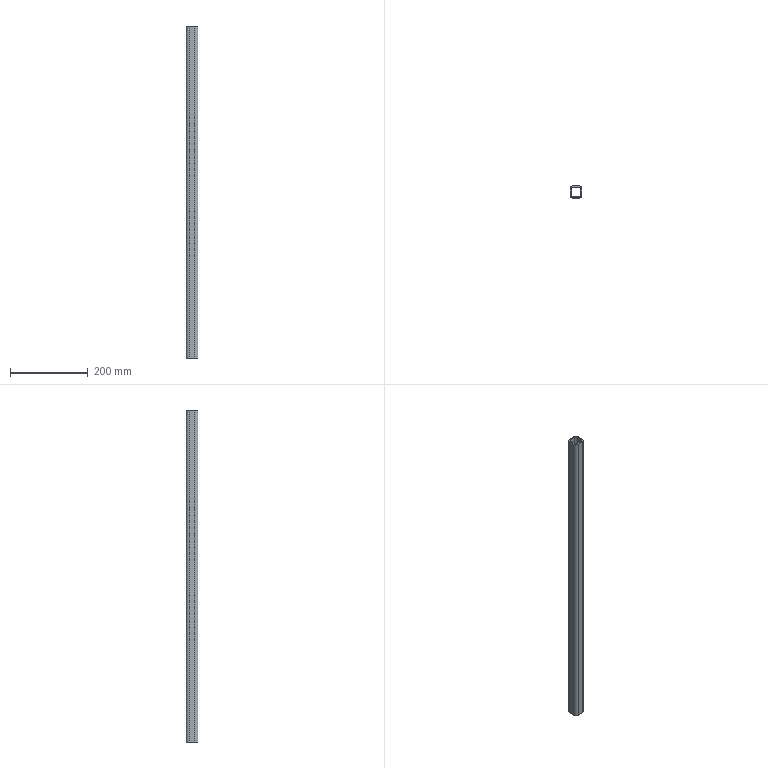Part | SolidWorks | features BaseBody 1 | 1 solid | 18 faces | box 30 x 30 x 852 mm | volume 249719 mm3 | plane 10 | cylinder 8 | commonest cylinder face diameters 9 x4 15 x4
STEP:
#1=CARTESIAN_POINT('',(7.5,-12.,0.));
#2=VERTEX_POINT('',#1);
#3=CARTESIAN_POINT('',(7.5,-12.,852.));
#4=VERTEX_POINT('',#3);
#5=CARTESIAN_POINT('',(7.5,-12.,0.));
#6=DIRECTION('',(0.,0.,1.));
#7=VECTOR('',#6,1000.);
#8=LINE('',#5,#7);
#9=EDGE_CURVE('',#2,#4,#8,.T.);
#10=ORIENTED_EDGE('',*,*,#9,.F.);
#11=CARTESIAN_POINT('',(-7.5,-12.,0.));
#12=VERTEX_POINT('',#11);
#13=CARTESIAN_POINT('',(7.5,-12.,0.));
#14=DIRECTION('',(1.,0.,0.));
#15=VECTOR('',#14,1000.);
#16=LINE('',#13,#15);
#17=EDGE_CURVE('',#12,#2,#16,.T.);
#18=ORIENTED_EDGE('',*,*,#17,.F.);
#19=CARTESIAN_POINT('',(-7.5,-12.,852.));
#20=VERTEX_POINT('',#19);
#21=CARTESIAN_POINT('',(-7.5,-12.,0.));
#22=DIRECTION('',(0.,0.,-1.));
#23=VECTOR('',#22,1000.);
#24=LINE('',#21,#23);
#25=EDGE_CURVE('',#20,#12,#24,.T.);
#26=ORIENTED_EDGE('',*,*,#25,.F.);
#27=CARTESIAN_POINT('',(7.5,-12.,852.));
#28=DIRECTION('',(-1.,0.,0.));
#29=VECTOR('',#28,1000.);
#30=LINE('',#27,#29);
#31=EDGE_CURVE('',#4,#20,#30,.T.);
#32=ORIENTED_EDGE('',*,*,#31,.F.);
#33=EDGE_LOOP('',(#10,#18,#26,#32));
#34=FACE_OUTER_BOUND('',#33,.T.);
#35=CARTESIAN_POINT('',(7.5,-12.,0.));
#36=DIRECTION('',(0.,-1.,0.));
#37=DIRECTION('',(1.,0.,0.));
#38=AXIS2_PLACEMENT_3D('',#35,#36,#37);
#39=PLANE('',#38);
#40=ADVANCED_FACE('',(#34),#39,.F.);
#41=CARTESIAN_POINT('',(-12.,-7.5,852.));
#42=VERTEX_POINT('',#41);
#43=CARTESIAN_POINT('',(-12.,7.5,852.));
#44=VERTEX_POINT('',#43);
#45=CARTESIAN_POINT('',(-12.,0.,852.));
#46=DIRECTION('',(0.,1.,0.));
#47=VECTOR('',#46,1000.);
#48=LINE('',#45,#47);
#49=EDGE_CURVE('',#42,#44,#48,.T.);
#50=ORIENTED_EDGE('',*,*,#49,.T.);
#51=CARTESIAN_POINT('',(-7.5,12.,852.));
#52=VERTEX_POINT('',#51);
#53=CARTESIAN_POINT('',(-7.5,7.5,852.));
#54=DIRECTION('',(0.,0.,-1.));
#55=DIRECTION('',(1.,0.,0.));
#56=AXIS2_PLACEMENT_3D('',#53,#54,#55);
#57=CIRCLE('',#56,4.5);
#58=EDGE_CURVE('',#44,#52,#57,.T.);
#59=ORIENTED_EDGE('',*,*,#58,.T.);
#60=CARTESIAN_POINT('',(7.5,12.,852.));
#61=VERTEX_POINT('',#60);
#62=CARTESIAN_POINT('',(0.,12.,852.));
#63=DIRECTION('',(1.,0.,0.));
#64=VECTOR('',#63,1000.);
#65=LINE('',#62,#64);
#66=EDGE_CURVE('',#52,#61,#65,.T.);
#67=ORIENTED_EDGE('',*,*,#66,.T.);
#68=CARTESIAN_POINT('',(12.,7.5,852.));
#69=VERTEX_POINT('',#68);
#70=CARTESIAN_POINT('',(7.5,7.5,852.));
#71=DIRECTION('',(0.,0.,-1.));
#72=DIRECTION('',(1.,0.,0.));
#73=AXIS2_PLACEMENT_3D('',#70,#71,#72);
#74=CIRCLE('',#73,4.5);
#75=EDGE_CURVE('',#61,#69,#74,.T.);
#76=ORIENTED_EDGE('',*,*,#75,.T.);
#77=CARTESIAN_POINT('',(12.,-7.5,852.));
#78=VERTEX_POINT('',#77);
#79=CARTESIAN_POINT('',(12.,0.,852.));
#80=DIRECTION('',(0.,-1.,0.));
#81=VECTOR('',#80,1000.);
#82=LINE('',#79,#81);
#83=EDGE_CURVE('',#69,#78,#82,.T.);
#84=ORIENTED_EDGE('',*,*,#83,.T.);
#85=CARTESIAN_POINT('',(7.5,-7.5,852.));
#86=DIRECTION('',(0.,0.,-1.));
#87=DIRECTION('',(1.,0.,0.));
#88=AXIS2_PLACEMENT_3D('',#85,#86,#87);
#89=CIRCLE('',#88,4.5);
#90=EDGE_CURVE('',#78,#4,#89,.T.);
#91=ORIENTED_EDGE('',*,*,#90,.T.);
#92=ORIENTED_EDGE('',*,*,#31,.T.);
#93=CARTESIAN_POINT('',(-7.5,-7.5,852.));
#94=DIRECTION('',(0.,0.,-1.));
#95=DIRECTION('',(1.,0.,0.));
#96=AXIS2_PLACEMENT_3D('',#93,#94,#95);
#97=CIRCLE('',#96,4.5);
#98=EDGE_CURVE('',#20,#42,#97,.T.);
#99=ORIENTED_EDGE('',*,*,#98,.T.);
#100=EDGE_LOOP('',(#50,#59,#67,#76,#84,#91,#92,#99));
#101=FACE_BOUND('',#100,.T.);
#102=CARTESIAN_POINT('',(7.5,15.,852.));
#103=VERTEX_POINT('',#102);
#104=CARTESIAN_POINT('',(-7.5,15.,852.));
#105=VERTEX_POINT('',#104);
#106=CARTESIAN_POINT('',(0.,15.,852.));
#107=DIRECTION('',(-1.,0.,0.));
#108=VECTOR('',#107,1000.);
#109=LINE('',#106,#108);
#110=EDGE_CURVE('',#103,#105,#109,.T.);
#111=ORIENTED_EDGE('',*,*,#110,.T.);
#112=CARTESIAN_POINT('',(-15.,7.5,852.));
#113=VERTEX_POINT('',#112);
#114=CARTESIAN_POINT('',(-7.5,7.5,852.));
#115=DIRECTION('',(0.,0.,1.));
#116=DIRECTION('',(1.,0.,0.));
#117=AXIS2_PLACEMENT_3D('',#114,#115,#116);
#118=CIRCLE('',#117,7.5);
#119=EDGE_CURVE('',#105,#113,#118,.T.);
#120=ORIENTED_EDGE('',*,*,#119,.T.);
#121=CARTESIAN_POINT('',(-15.,-7.5,852.));
#122=VERTEX_POINT('',#121);
#123=CARTESIAN_POINT('',(-15.,0.,852.));
#124=DIRECTION('',(0.,-1.,0.));
#125=VECTOR('',#124,1000.);
#126=LINE('',#123,#125);
#127=EDGE_CURVE('',#113,#122,#126,.T.);
#128=ORIENTED_EDGE('',*,*,#127,.T.);
#129=CARTESIAN_POINT('',(-7.5,-15.,852.));
#130=VERTEX_POINT('',#129);
#131=CARTESIAN_POINT('',(-7.5,-7.5,852.));
#132=DIRECTION('',(0.,0.,1.));
#133=DIRECTION('',(1.,0.,0.));
#134=AXIS2_PLACEMENT_3D('',#131,#132,#133);
#135=CIRCLE('',#134,7.5);
#136=EDGE_CURVE('',#122,#130,#135,.T.);
#137=ORIENTED_EDGE('',*,*,#136,.T.);
#138=CARTESIAN_POINT('',(7.5,-15.,852.));
#139=VERTEX_POINT('',#138);
#140=CARTESIAN_POINT('',(0.,-15.,852.));
#141=DIRECTION('',(1.,0.,0.));
#142=VECTOR('',#141,1000.);
#143=LINE('',#140,#142);
#144=EDGE_CURVE('',#130,#139,#143,.T.);
#145=ORIENTED_EDGE('',*,*,#144,.T.);
#146=CARTESIAN_POINT('',(15.,-7.5,852.));
#147=VERTEX_POINT('',#146);
#148=CARTESIAN_POINT('',(7.5,-7.5,852.));
#149=DIRECTION('',(0.,0.,1.));
#150=DIRECTION('',(1.,0.,0.));
#151=AXIS2_PLACEMENT_3D('',#148,#149,#150);
#152=CIRCLE('',#151,7.5);
#153=EDGE_CURVE('',#139,#147,#152,.T.);
#154=ORIENTED_EDGE('',*,*,#153,.T.);
#155=CARTESIAN_POINT('',(15.,7.5,852.));
#156=VERTEX_POINT('',#155);
#157=CARTESIAN_POINT('',(15.,0.,852.));
#158=DIRECTION('',(0.,1.,0.));
#159=VECTOR('',#158,1000.);
#160=LINE('',#157,#159);
#161=EDGE_CURVE('',#147,#156,#160,.T.);
#162=ORIENTED_EDGE('',*,*,#161,.T.);
#163=CARTESIAN_POINT('',(7.5,7.5,852.));
#164=DIRECTION('',(0.,0.,1.));
#165=DIRECTION('',(1.,0.,0.));
#166=AXIS2_PLACEMENT_3D('',#163,#164,#165);
#167=CIRCLE('',#166,7.5);
#168=EDGE_CURVE('',#156,#103,#167,.T.);
#169=ORIENTED_EDGE('',*,*,#168,.T.);
#170=EDGE_LOOP('',(#111,#120,#128,#137,#145,#154,#162,#169));
#171=FACE_OUTER_BOUND('',#170,.T.);
#172=CARTESIAN_POINT('',(0.,0.,852.));
#173=DIRECTION('',(0.,0.,1.));
#174=DIRECTION('',(1.,0.,0.));
#175=AXIS2_PLACEMENT_3D('',#172,#173,#174);
#176=PLANE('',#175);
#177=ADVANCED_FACE('',(#101,#171),#176,.T.);
#178=CARTESIAN_POINT('',(12.,-7.5,0.));
#179=VERTEX_POINT('',#178);
#180=CARTESIAN_POINT('',(12.,-7.5,0.));
#181=DIRECTION('',(0.,0.,1.));
#182=VECTOR('',#181,1000.);
#183=LINE('',#180,#182);
#184=EDGE_CURVE('',#179,#78,#183,.T.);
#185=ORIENTED_EDGE('',*,*,#184,.F.);
#186=CARTESIAN_POINT('',(7.5,-7.5,0.));
#187=DIRECTION('',(0.,0.,1.));
#188=DIRECTION('',(1.,0.,0.));
#189=AXIS2_PLACEMENT_3D('',#186,#187,#188);
#190=CIRCLE('',#189,4.5);
#191=EDGE_CURVE('',#2,#179,#190,.T.);
#192=ORIENTED_EDGE('',*,*,#191,.F.);
#193=ORIENTED_EDGE('',*,*,#9,.T.);
#194=ORIENTED_EDGE('',*,*,#90,.F.);
#195=EDGE_LOOP('',(#185,#192,#193,#194));
#196=FACE_OUTER_BOUND('',#195,.T.);
#197=CARTESIAN_POINT('',(7.5,-7.5,0.));
#198=DIRECTION('',(0.,0.,1.));
#199=DIRECTION('',(1.,0.,0.));
#200=AXIS2_PLACEMENT_3D('',#197,#198,#199);
#201=CYLINDRICAL_SURFACE('',#200,4.5);
#202=ADVANCED_FACE('',(#196),#201,.F.);
#203=CARTESIAN_POINT('',(-12.,7.5,0.));
#204=VERTEX_POINT('',#203);
#205=CARTESIAN_POINT('',(-7.5,12.,0.));
#206=VERTEX_POINT('',#205);
#207=CARTESIAN_POINT('',(-7.5,7.5,0.));
#208=DIRECTION('',(0.,0.,-1.));
#209=DIRECTION('',(1.,0.,0.));
#210=AXIS2_PLACEMENT_3D('',#207,#208,#209);
#211=CIRCLE('',#210,4.5);
#212=EDGE_CURVE('',#204,#206,#211,.T.);
#213=ORIENTED_EDGE('',*,*,#212,.F.);
#214=CARTESIAN_POINT('',(-12.,-7.5,0.));
#215=VERTEX_POINT('',#214);
#216=CARTESIAN_POINT('',(-12.,0.,0.));
#217=DIRECTION('',(0.,1.,0.));
#218=VECTOR('',#217,1000.);
#219=LINE('',#216,#218);
#220=EDGE_CURVE('',#215,#204,#219,.T.);
#221=ORIENTED_EDGE('',*,*,#220,.F.);
#222=CARTESIAN_POINT('',(-7.5,-7.5,0.));
#223=DIRECTION('',(0.,0.,-1.));
#224=DIRECTION('',(1.,0.,0.));
#225=AXIS2_PLACEMENT_3D('',#222,#223,#224);
#226=CIRCLE('',#225,4.5);
#227=EDGE_CURVE('',#12,#215,#226,.T.);
#228=ORIENTED_EDGE('',*,*,#227,.F.);
#229=ORIENTED_EDGE('',*,*,#17,.T.);
#230=ORIENTED_EDGE('',*,*,#191,.T.);
#231=CARTESIAN_POINT('',(12.,7.5,0.));
#232=VERTEX_POINT('',#231);
#233=CARTESIAN_POINT('',(12.,0.,0.));
#234=DIRECTION('',(0.,-1.,0.));
#235=VECTOR('',#234,1000.);
#236=LINE('',#233,#235);
#237=EDGE_CURVE('',#232,#179,#236,.T.);
#238=ORIENTED_EDGE('',*,*,#237,.F.);
#239=CARTESIAN_POINT('',(7.5,12.,0.));
#240=VERTEX_POINT('',#239);
#241=CARTESIAN_POINT('',(7.5,7.5,0.));
#242=DIRECTION('',(0.,0.,-1.));
#243=DIRECTION('',(1.,0.,0.));
#244=AXIS2_PLACEMENT_3D('',#241,#242,#243);
#245=CIRCLE('',#244,4.5);
#246=EDGE_CURVE('',#240,#232,#245,.T.);
#247=ORIENTED_EDGE('',*,*,#246,.F.);
#248=CARTESIAN_POINT('',(0.,12.,0.));
#249=DIRECTION('',(1.,0.,0.));
#250=VECTOR('',#249,1000.);
#251=LINE('',#248,#250);
#252=EDGE_CURVE('',#206,#240,#251,.T.);
#253=ORIENTED_EDGE('',*,*,#252,.F.);
#254=EDGE_LOOP('',(#213,#221,#228,#229,#230,#238,#247,#253));
#255=FACE_BOUND('',#254,.T.);
#256=CARTESIAN_POINT('',(-7.5,15.,0.));
#257=VERTEX_POINT('',#256);
#258=CARTESIAN_POINT('',(-15.,7.5,0.));
#259=VERTEX_POINT('',#258);
#260=CARTESIAN_POINT('',(-7.5,7.5,0.));
#261=DIRECTION('',(0.,0.,1.));
#262=DIRECTION('',(1.,0.,0.));
#263=AXIS2_PLACEMENT_3D('',#260,#261,#262);
#264=CIRCLE('',#263,7.5);
#265=EDGE_CURVE('',#257,#259,#264,.T.);
#266=ORIENTED_EDGE('',*,*,#265,.F.);
#267=CARTESIAN_POINT('',(7.5,15.,0.));
#268=VERTEX_POINT('',#267);
#269=CARTESIAN_POINT('',(0.,15.,0.));
#270=DIRECTION('',(-1.,0.,0.));
#271=VECTOR('',#270,1000.);
#272=LINE('',#269,#271);
#273=EDGE_CURVE('',#268,#257,#272,.T.);
#274=ORIENTED_EDGE('',*,*,#273,.F.);
#275=CARTESIAN_POINT('',(15.,7.5,0.));
#276=VERTEX_POINT('',#275);
#277=CARTESIAN_POINT('',(7.5,7.5,0.));
#278=DIRECTION('',(0.,0.,1.));
#279=DIRECTION('',(1.,0.,0.));
#280=AXIS2_PLACEMENT_3D('',#277,#278,#279);
#281=CIRCLE('',#280,7.5);
#282=EDGE_CURVE('',#276,#268,#281,.T.);
#283=ORIENTED_EDGE('',*,*,#282,.F.);
#284=CARTESIAN_POINT('',(15.,-7.5,0.));
#285=VERTEX_POINT('',#284);
#286=CARTESIAN_POINT('',(15.,0.,0.));
#287=DIRECTION('',(0.,1.,0.));
#288=VECTOR('',#287,1000.);
#289=LINE('',#286,#288);
#290=EDGE_CURVE('',#285,#276,#289,.T.);
#291=ORIENTED_EDGE('',*,*,#290,.F.);
#292=CARTESIAN_POINT('',(7.5,-15.,0.));
#293=VERTEX_POINT('',#292);
#294=CARTESIAN_POINT('',(7.5,-7.5,0.));
#295=DIRECTION('',(0.,0.,1.));
#296=DIRECTION('',(1.,0.,0.));
#297=AXIS2_PLACEMENT_3D('',#294,#295,#296);
#298=CIRCLE('',#297,7.5);
#299=EDGE_CURVE('',#293,#285,#298,.T.);
#300=ORIENTED_EDGE('',*,*,#299,.F.);
#301=CARTESIAN_POINT('',(-7.5,-15.,0.));
#302=VERTEX_POINT('',#301);
#303=CARTESIAN_POINT('',(0.,-15.,0.));
#304=DIRECTION('',(1.,0.,0.));
#305=VECTOR('',#304,1000.);
#306=LINE('',#303,#305);
#307=EDGE_CURVE('',#302,#293,#306,.T.);
#308=ORIENTED_EDGE('',*,*,#307,.F.);
#309=CARTESIAN_POINT('',(-15.,-7.5,0.));
#310=VERTEX_POINT('',#309);
#311=CARTESIAN_POINT('',(-7.5,-7.5,0.));
#312=DIRECTION('',(0.,0.,1.));
#313=DIRECTION('',(1.,0.,0.));
#314=AXIS2_PLACEMENT_3D('',#311,#312,#313);
#315=CIRCLE('',#314,7.5);
#316=EDGE_CURVE('',#310,#302,#315,.T.);
#317=ORIENTED_EDGE('',*,*,#316,.F.);
#318=CARTESIAN_POINT('',(-15.,0.,0.));
#319=DIRECTION('',(0.,-1.,0.));
#320=VECTOR('',#319,1000.);
#321=LINE('',#318,#320);
#322=EDGE_CURVE('',#259,#310,#321,.T.);
#323=ORIENTED_EDGE('',*,*,#322,.F.);
#324=EDGE_LOOP('',(#266,#274,#283,#291,#300,#308,#317,#323));
#325=FACE_OUTER_BOUND('',#324,.T.);
#326=CARTESIAN_POINT('',(0.,0.,0.));
#327=DIRECTION('',(0.,0.,1.));
#328=DIRECTION('',(1.,0.,0.));
#329=AXIS2_PLACEMENT_3D('',#326,#327,#328);
#330=PLANE('',#329);
#331=ADVANCED_FACE('',(#255,#325),#330,.F.);
#332=ORIENTED_EDGE('',*,*,#25,.T.);
#333=ORIENTED_EDGE('',*,*,#227,.T.);
#334=CARTESIAN_POINT('',(-12.,-7.5,0.));
#335=DIRECTION('',(0.,0.,-1.));
#336=VECTOR('',#335,1000.);
#337=LINE('',#334,#336);
#338=EDGE_CURVE('',#42,#215,#337,.T.);
#339=ORIENTED_EDGE('',*,*,#338,.F.);
#340=ORIENTED_EDGE('',*,*,#98,.F.);
#341=EDGE_LOOP('',(#332,#333,#339,#340));
#342=FACE_OUTER_BOUND('',#341,.T.);
#343=CARTESIAN_POINT('',(-7.5,-7.5,0.));
#344=DIRECTION('',(0.,0.,1.));
#345=DIRECTION('',(1.,0.,0.));
#346=AXIS2_PLACEMENT_3D('',#343,#344,#345);
#347=CYLINDRICAL_SURFACE('',#346,4.5);
#348=ADVANCED_FACE('',(#342),#347,.F.);
#349=CARTESIAN_POINT('',(-12.,7.5,0.));
#350=DIRECTION('',(0.,0.,1.));
#351=VECTOR('',#350,1000.);
#352=LINE('',#349,#351);
#353=EDGE_CURVE('',#204,#44,#352,.T.);
#354=ORIENTED_EDGE('',*,*,#353,.F.);
#355=ORIENTED_EDGE('',*,*,#212,.T.);
#356=CARTESIAN_POINT('',(-7.5,12.,0.));
#357=DIRECTION('',(0.,0.,-1.));
#358=VECTOR('',#357,1000.);
#359=LINE('',#356,#358);
#360=EDGE_CURVE('',#52,#206,#359,.T.);
#361=ORIENTED_EDGE('',*,*,#360,.F.);
#362=ORIENTED_EDGE('',*,*,#58,.F.);
#363=EDGE_LOOP('',(#354,#355,#361,#362));
#364=FACE_OUTER_BOUND('',#363,.T.);
#365=CARTESIAN_POINT('',(-7.5,7.5,0.));
#366=DIRECTION('',(0.,0.,1.));
#367=DIRECTION('',(1.,0.,0.));
#368=AXIS2_PLACEMENT_3D('',#365,#366,#367);
#369=CYLINDRICAL_SURFACE('',#368,4.5);
#370=ADVANCED_FACE('',(#364),#369,.F.);
#371=ORIENTED_EDGE('',*,*,#338,.T.);
#372=ORIENTED_EDGE('',*,*,#220,.T.);
#373=ORIENTED_EDGE('',*,*,#353,.T.);
#374=ORIENTED_EDGE('',*,*,#49,.F.);
#375=EDGE_LOOP('',(#371,#372,#373,#374));
#376=FACE_OUTER_BOUND('',#375,.T.);
#377=CARTESIAN_POINT('',(-12.,-7.5,0.));
#378=DIRECTION('',(-1.,0.,0.));
#379=DIRECTION('',(0.,-1.,0.));
#380=AXIS2_PLACEMENT_3D('',#377,#378,#379);
#381=PLANE('',#380);
#382=ADVANCED_FACE('',(#376),#381,.F.);
#383=CARTESIAN_POINT('',(12.,7.5,0.));
#384=DIRECTION('',(0.,0.,1.));
#385=VECTOR('',#384,1000.);
#386=LINE('',#383,#385);
#387=EDGE_CURVE('',#232,#69,#386,.T.);
#388=ORIENTED_EDGE('',*,*,#387,.F.);
#389=ORIENTED_EDGE('',*,*,#237,.T.);
#390=ORIENTED_EDGE('',*,*,#184,.T.);
#391=ORIENTED_EDGE('',*,*,#83,.F.);
#392=EDGE_LOOP('',(#388,#389,#390,#391));
#393=FACE_OUTER_BOUND('',#392,.T.);
#394=CARTESIAN_POINT('',(12.,7.5,0.));
#395=DIRECTION('',(1.,0.,0.));
#396=DIRECTION('',(0.,0.,-1.));
#397=AXIS2_PLACEMENT_3D('',#394,#395,#396);
#398=PLANE('',#397);
#399=ADVANCED_FACE('',(#393),#398,.F.);
#400=CARTESIAN_POINT('',(7.5,12.,0.));
#401=DIRECTION('',(0.,0.,1.));
#402=VECTOR('',#401,1000.);
#403=LINE('',#400,#402);
#404=EDGE_CURVE('',#240,#61,#403,.T.);
#405=ORIENTED_EDGE('',*,*,#404,.F.);
#406=ORIENTED_EDGE('',*,*,#246,.T.);
#407=ORIENTED_EDGE('',*,*,#387,.T.);
#408=ORIENTED_EDGE('',*,*,#75,.F.);
#409=EDGE_LOOP('',(#405,#406,#407,#408));
#410=FACE_OUTER_BOUND('',#409,.T.);
#411=CARTESIAN_POINT('',(7.5,7.5,0.));
#412=DIRECTION('',(0.,0.,1.));
#413=DIRECTION('',(1.,0.,0.));
#414=AXIS2_PLACEMENT_3D('',#411,#412,#413);
#415=CYLINDRICAL_SURFACE('',#414,4.5);
#416=ADVANCED_FACE('',(#410),#415,.F.);
#417=ORIENTED_EDGE('',*,*,#360,.T.);
#418=ORIENTED_EDGE('',*,*,#252,.T.);
#419=ORIENTED_EDGE('',*,*,#404,.T.);
#420=ORIENTED_EDGE('',*,*,#66,.F.);
#421=EDGE_LOOP('',(#417,#418,#419,#420));
#422=FACE_OUTER_BOUND('',#421,.T.);
#423=CARTESIAN_POINT('',(-7.5,12.,0.));
#424=DIRECTION('',(0.,1.,0.));
#425=DIRECTION('',(-1.,0.,0.));
#426=AXIS2_PLACEMENT_3D('',#423,#424,#425);
#427=PLANE('',#426);
#428=ADVANCED_FACE('',(#422),#427,.F.);
#429=ORIENTED_EDGE('',*,*,#265,.T.);
#430=CARTESIAN_POINT('',(-15.,7.5,0.));
#431=DIRECTION('',(0.,0.,1.));
#432=VECTOR('',#431,1000.);
#433=LINE('',#430,#432);
#434=EDGE_CURVE('',#259,#113,#433,.T.);
#435=ORIENTED_EDGE('',*,*,#434,.T.);
#436=ORIENTED_EDGE('',*,*,#119,.F.);
#437=CARTESIAN_POINT('',(-7.5,15.,0.));
#438=DIRECTION('',(0.,0.,-1.));
#439=VECTOR('',#438,1000.);
#440=LINE('',#437,#439);
#441=EDGE_CURVE('',#105,#257,#440,.T.);
#442=ORIENTED_EDGE('',*,*,#441,.T.);
#443=EDGE_LOOP('',(#429,#435,#436,#442));
#444=FACE_OUTER_BOUND('',#443,.T.);
#445=CARTESIAN_POINT('',(-7.5,7.5,0.));
#446=DIRECTION('',(0.,0.,1.));
#447=DIRECTION('',(1.,0.,0.));
#448=AXIS2_PLACEMENT_3D('',#445,#446,#447);
#449=CYLINDRICAL_SURFACE('',#448,7.5);
#450=ADVANCED_FACE('',(#444),#449,.T.);
#451=ORIENTED_EDGE('',*,*,#273,.T.);
#452=ORIENTED_EDGE('',*,*,#441,.F.);
#453=ORIENTED_EDGE('',*,*,#110,.F.);
#454=CARTESIAN_POINT('',(7.5,15.,0.));
#455=DIRECTION('',(0.,0.,-1.));
#456=VECTOR('',#455,1000.);
#457=LINE('',#454,#456);
#458=EDGE_CURVE('',#103,#268,#457,.T.);
#459=ORIENTED_EDGE('',*,*,#458,.T.);
#460=EDGE_LOOP('',(#451,#452,#453,#459));
#461=FACE_OUTER_BOUND('',#460,.T.);
#462=CARTESIAN_POINT('',(-7.5,15.,0.));
#463=DIRECTION('',(0.,1.,0.));
#464=DIRECTION('',(-1.,0.,0.));
#465=AXIS2_PLACEMENT_3D('',#462,#463,#464);
#466=PLANE('',#465);
#467=ADVANCED_FACE('',(#461),#466,.T.);
#468=ORIENTED_EDGE('',*,*,#282,.T.);
#469=ORIENTED_EDGE('',*,*,#458,.F.);
#470=ORIENTED_EDGE('',*,*,#168,.F.);
#471=CARTESIAN_POINT('',(15.,7.5,0.));
#472=DIRECTION('',(0.,0.,-1.));
#473=VECTOR('',#472,1000.);
#474=LINE('',#471,#473);
#475=EDGE_CURVE('',#156,#276,#474,.T.);
#476=ORIENTED_EDGE('',*,*,#475,.T.);
#477=EDGE_LOOP('',(#468,#469,#470,#476));
#478=FACE_OUTER_BOUND('',#477,.T.);
#479=CARTESIAN_POINT('',(7.5,7.5,0.));
#480=DIRECTION('',(0.,0.,1.));
#481=DIRECTION('',(1.,0.,0.));
#482=AXIS2_PLACEMENT_3D('',#479,#480,#481);
#483=CYLINDRICAL_SURFACE('',#482,7.5);
#484=ADVANCED_FACE('',(#478),#483,.T.);
#485=ORIENTED_EDGE('',*,*,#290,.T.);
#486=ORIENTED_EDGE('',*,*,#475,.F.);
#487=ORIENTED_EDGE('',*,*,#161,.F.);
#488=CARTESIAN_POINT('',(15.,-7.5,0.));
#489=DIRECTION('',(0.,0.,-1.));
#490=VECTOR('',#489,1000.);
#491=LINE('',#488,#490);
#492=EDGE_CURVE('',#147,#285,#491,.T.);
#493=ORIENTED_EDGE('',*,*,#492,.T.);
#494=EDGE_LOOP('',(#485,#486,#487,#493));
#495=FACE_OUTER_BOUND('',#494,.T.);
#496=CARTESIAN_POINT('',(15.,7.5,0.));
#497=DIRECTION('',(1.,0.,0.));
#498=DIRECTION('',(0.,1.,0.));
#499=AXIS2_PLACEMENT_3D('',#496,#497,#498);
#500=PLANE('',#499);
#501=ADVANCED_FACE('',(#495),#500,.T.);
#502=ORIENTED_EDGE('',*,*,#299,.T.);
#503=ORIENTED_EDGE('',*,*,#492,.F.);
#504=ORIENTED_EDGE('',*,*,#153,.F.);
#505=CARTESIAN_POINT('',(7.5,-15.,0.));
#506=DIRECTION('',(0.,0.,-1.));
#507=VECTOR('',#506,1000.);
#508=LINE('',#505,#507);
#509=EDGE_CURVE('',#139,#293,#508,.T.);
#510=ORIENTED_EDGE('',*,*,#509,.T.);
#511=EDGE_LOOP('',(#502,#503,#504,#510));
#512=FACE_OUTER_BOUND('',#511,.T.);
#513=CARTESIAN_POINT('',(7.5,-7.5,0.));
#514=DIRECTION('',(0.,0.,1.));
#515=DIRECTION('',(1.,0.,0.));
#516=AXIS2_PLACEMENT_3D('',#513,#514,#515);
#517=CYLINDRICAL_SURFACE('',#516,7.5);
#518=ADVANCED_FACE('',(#512),#517,.T.);
#519=ORIENTED_EDGE('',*,*,#307,.T.);
#520=ORIENTED_EDGE('',*,*,#509,.F.);
#521=ORIENTED_EDGE('',*,*,#144,.F.);
#522=CARTESIAN_POINT('',(-7.5,-15.,0.));
#523=DIRECTION('',(0.,0.,-1.));
#524=VECTOR('',#523,1000.);
#525=LINE('',#522,#524);
#526=EDGE_CURVE('',#130,#302,#525,.T.);
#527=ORIENTED_EDGE('',*,*,#526,.T.);
#528=EDGE_LOOP('',(#519,#520,#521,#527));
#529=FACE_OUTER_BOUND('',#528,.T.);
#530=CARTESIAN_POINT('',(7.5,-15.,0.));
#531=DIRECTION('',(0.,-1.,0.));
#532=DIRECTION('',(1.,0.,0.));
#533=AXIS2_PLACEMENT_3D('',#530,#531,#532);
#534=PLANE('',#533);
#535=ADVANCED_FACE('',(#529),#534,.T.);
#536=ORIENTED_EDGE('',*,*,#316,.T.);
#537=ORIENTED_EDGE('',*,*,#526,.F.);
#538=ORIENTED_EDGE('',*,*,#136,.F.);
#539=CARTESIAN_POINT('',(-15.,-7.5,0.));
#540=DIRECTION('',(0.,0.,-1.));
#541=VECTOR('',#540,1000.);
#542=LINE('',#539,#541);
#543=EDGE_CURVE('',#122,#310,#542,.T.);
#544=ORIENTED_EDGE('',*,*,#543,.T.);
#545=EDGE_LOOP('',(#536,#537,#538,#544));
#546=FACE_OUTER_BOUND('',#545,.T.);
#547=CARTESIAN_POINT('',(-7.5,-7.5,0.));
#548=DIRECTION('',(0.,0.,1.));
#549=DIRECTION('',(1.,0.,0.));
#550=AXIS2_PLACEMENT_3D('',#547,#548,#549);
#551=CYLINDRICAL_SURFACE('',#550,7.5);
#552=ADVANCED_FACE('',(#546),#551,.T.);
#553=ORIENTED_EDGE('',*,*,#322,.T.);
#554=ORIENTED_EDGE('',*,*,#543,.F.);
#555=ORIENTED_EDGE('',*,*,#127,.F.);
#556=ORIENTED_EDGE('',*,*,#434,.F.);
#557=EDGE_LOOP('',(#553,#554,#555,#556));
#558=FACE_OUTER_BOUND('',#557,.T.);
#559=CARTESIAN_POINT('',(-15.,-7.5,0.));
#560=DIRECTION('',(-1.,0.,0.));
#561=DIRECTION('',(0.,0.,1.));
#562=AXIS2_PLACEMENT_3D('',#559,#560,#561);
#563=PLANE('',#562);
#564=ADVANCED_FACE('',(#558),#563,.T.);
#565=CLOSED_SHELL('',(#40,#177,#202,#331,#348,#370,#382,#399,#416,#428,#450,#467,#484,#501,#518,#535,#552,#564));
#566=MANIFOLD_SOLID_BREP('',#565);
#567=CARTESIAN_POINT('',(0.,0.,0.));
#568=DIRECTION('',(0.,0.,1.));
#569=DIRECTION('',(1.,0.,0.));
#570=AXIS2_PLACEMENT_3D('',#567,#568,#569);
#571=(LENGTH_UNIT()NAMED_UNIT(*)SI_UNIT(.MILLI.,.METRE.));
#572=UNCERTAINTY_MEASURE_WITH_UNIT(LENGTH_MEASURE(0.00001),#571,'','');
#573=(NAMED_UNIT(*)PLANE_ANGLE_UNIT()SI_UNIT($,.RADIAN.));
#574=(NAMED_UNIT(*)SI_UNIT($,.STERADIAN.)SOLID_ANGLE_UNIT());
#575=(GEOMETRIC_REPRESENTATION_CONTEXT(3)GLOBAL_UNCERTAINTY_ASSIGNED_CONTEXT((#572))GLOBAL_UNIT_ASSIGNED_CONTEXT((#571,#573,#574))REPRESENTATION_CONTEXT('',''));
#576=ADVANCED_BREP_SHAPE_REPRESENTATION('',(#566,#570),#575);